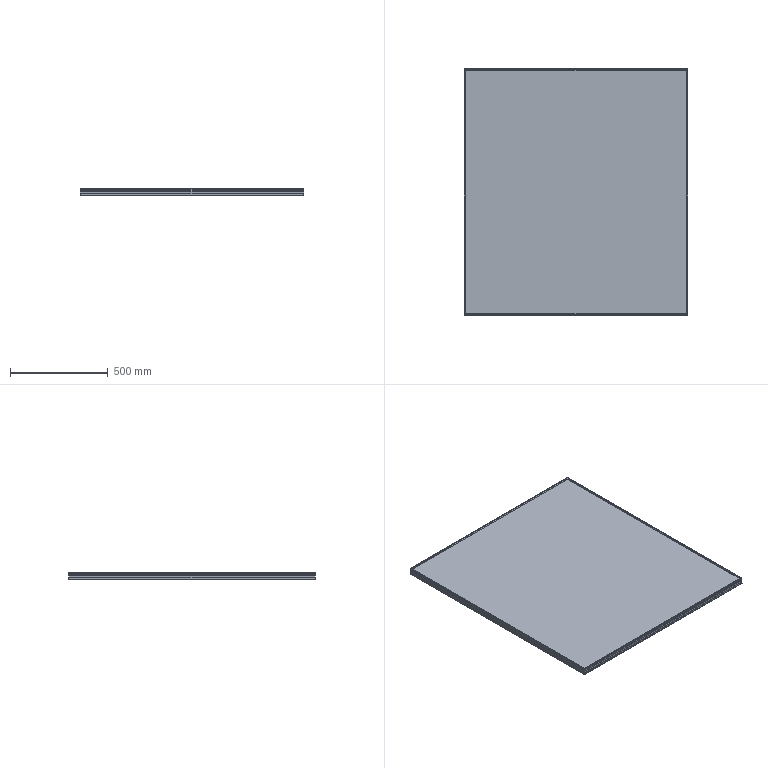Part | SolidWorks | 6 solids | 202 faces | box 1140 x 1260 x 36 mm | volume 6158512 mm3 | plane 148 | cylinder 54 | commonest cylinder face diameters 7 x50 5 x4